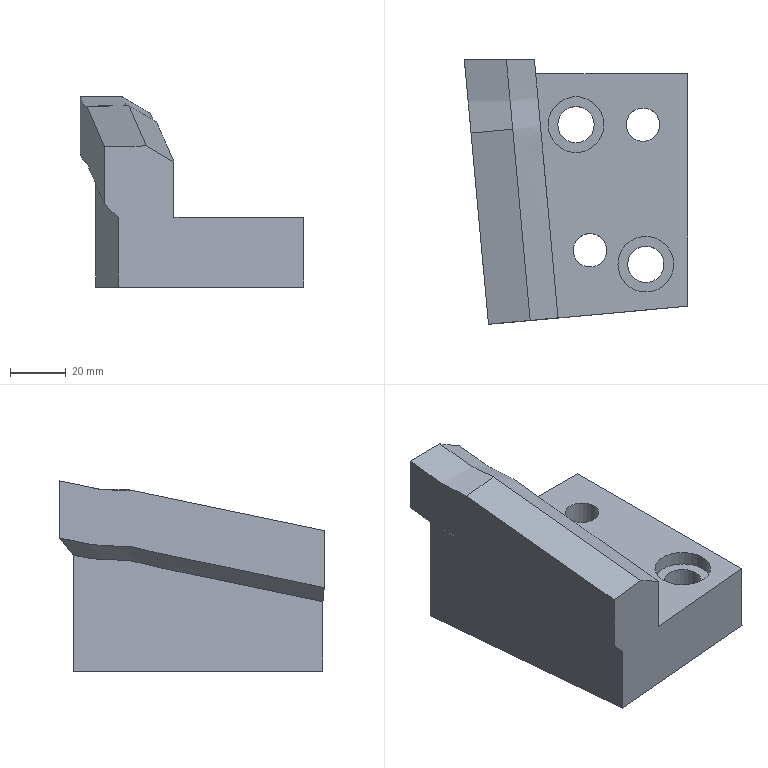Part | NX | features solid 2 | 1 solid | 22 faces | box 80 x 94.728 x 68.12 mm | volume 209715 mm3 | plane 9 | spline 7 | cylinder 6 | commonest cylinder face diameters 12 x2 13 x2 20 x2